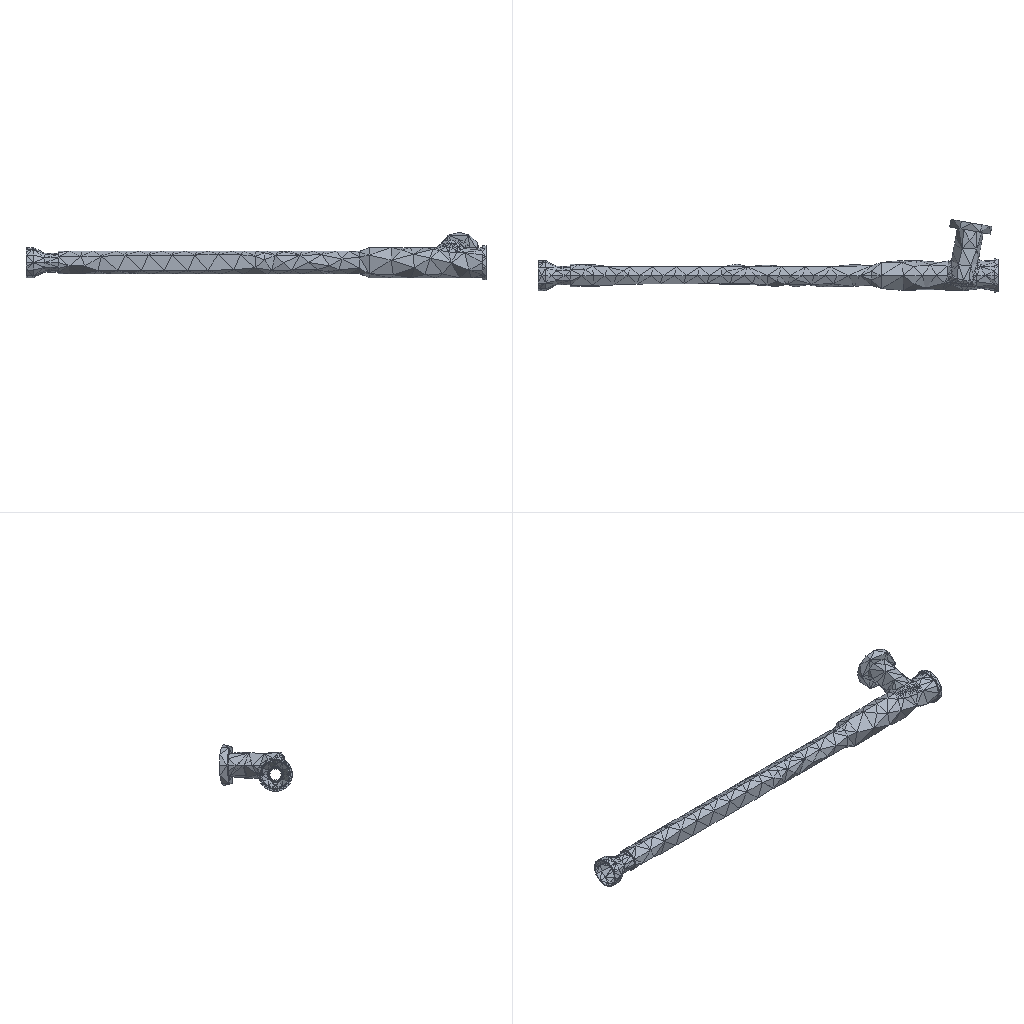Simulation study | ansys workbench
Ansys APDL input file, long lists of numbers shortened:
/batch
/config,noeldb,1     ! force off writing results to database
*get,_wallstrt,active,,time,wall
! ANSYS input file written by Workbench version 2022 R1
! File used for geometry attach: F:\ansys（分析文件汇总)\ansys转向器有限元分析\转向器\分析\齿轮轴.STEP
/title,wbnew--__ (C5)
! ****** Begin Custom Load Command Snippet ******
/COM, ACT Extensions:
/COM,     LSDYNA, 2021.1
/COM,
! ****** End   Custom Load Command Snippet ******
*DIM,_wb_ProjectScratch_dir,string,248
_wb_ProjectScratch_dir(1) = 'C:\Users\Administrator\AppData\Local\Temp\WB_Administrator_18756_2\_ProjectScratch\Scr9CF5\'
*DIM,_wb_SolverFiles_dir,string,248
_wb_SolverFiles_dir(1) = 'C:\Users\Administrator\AppData\Local\Temp\WB_Administrator_18756_2\wbnew_files\dp0\SYS-4\MECH\'
*DIM,_wb_userfiles_dir,string,248
_wb_userfiles_dir(1) = 'C:\Users\Administrator\AppData\Local\Temp\WB_Administrator_18756_2\wbnew_files\user_files\'
/com,--- Data in consistent NMM units. See Solving Units in the help system for more information.
/units,MPA
/nopr
/wb,file,start              !  signify a WB generated input file
/prep7
! Turn off shape checking because checks already performed inside WB mesher.
! See help system for more information.
SHPP,OFF,,NOWARN
/nolist
etcon,set             ! allow ANSYS to choose best KEYOP's for 180x elements, resets any applicable keyopt to MAPDL defaults
/com,*********** Nodes for the whole assembly ***********
nblock,3,,14898
(1i9,3e20.9e3)
        1     0.000000000E+00     1.290000000E+02    -2.000000000E+01
! (13543 more lines like these left out)
-1
/com,*********** Nodes for all Remote Points ***********
nblock,3
(1i9,3e20.9e3)
    13545    -4.024558464E-16     1.874095711E+02     4.440892099E-16
-1
/wb,elem,start            !  set before creation of elements
/com,*********** Elements for Body 1 "___-FreeParts|__-__1" ***********
et,1,187
eblock,19,solid,,7138
(19i9)
        1        1        1        1        0        0        0        0       10        0        1     1930     2216     2013     2164    12446    12852    12443    12445
! (14275 more lines like these left out)
-1
/wb,elem,end               !  done creating elements
/com,*********** Send User Defined Coordinate System(s) ***********
csys,0
toffst,273.15,  ! Temperature offset from absolute zero
/com,*********** Set Reference Temperature ***********
tref,22.
/wb,mat,start              !  starting to send materials
/com,*********** Send Materials ***********
Temperature = 'TEMP' ! Temperature
MP,DENS,1,7.85e-09,	! tonne mm^-3
MP,ALPX,1,1.2e-05,	! C^-1
MP,C,1,434000000,	! mm^2 s^-2 C^-1
MP,KXX,1,60.5,	! tonne mm s^-3 C^-1
MP,RSVX,1,0.00017,	! ohm mm
MP,EX,1,200000,	! tonne s^-2 mm^-1
MP,NUXY,1,0.3,
MP,MURX,1,10000,
/wb,mat,end                !  done sending materials
!************************* Model Summary ********************
!___-FreeParts|__-__1,	结构钢,	matid,	1
!************************* End Model Summary ********************
! get the diagonal of the bounding box. Needed later for other things
*get,_xmin,node,,mnloc,x
*get,_ymin,node,,mnloc,y
*get,_zmin,node,,mnloc,z
*get,_xmax,node,,mxloc,x
*get,_ymax,node,,mxloc,y
*get,_zmax,node,,mxloc,z
_ASMDIAG=(_xmax-_xmin)*(_xmax-_xmin)+(_ymax-_ymin)*(_ymax-_ymin)+(_zmax-_zmin)*(_zmax-_zmin)
_ASMDIAG=SQRT(_ASMDIAG)
/wb,contact,start          !  starting to send contact
/wb,contact,end            !  done creating contacts
/com,*********** Send Named Selection as Node Component ***********
CMBLOCK,______  ,NODE,     4510
(8i10)
        56        57        58        59        60        61        62        63
! (563 more lines like these left out)
/golist
/wb,load,start             !  starting to send loads
/gst,on,on
fini
*get,_numnode,node,0,count
*get,_numelem,elem,0,count
*get, _MAXELEMNUM, elem, 0, NUM, MAX
*get, _MAXNODENUM, node, 0, NUM, MAX
*get, _MAXELEMTYPE, etyp, 0, NUM, MAX
*get, _MAXREALCONST, real, 0, NUM, MAX
/go
/wb,load,end               !  done creating loads
/com,--- Number of total nodes = %_numnode%
/com,--- Number of contact elements = 0
/com,--- Number of spring elements = 0
/com,--- Number of bearing elements = 0
/com,--- Number of solid elements = 7138
/com,--- Number of condensed parts = 0
/com,--- Number of total elements = %_numelem%
*get,_wallbsol,active,,time,wall
/solu
antype,2                   ! modal analysis
_thickRatio=  1     ! Ratio of thick parts in the model
modopt,lanb,6
outres,erase
outres,all,none
outres,nsol,all
outres,etmp,all
mxpand                    ! default expand in case of complex solution
dmpopt,esav,no
dmpopt,emat,no
dmpopt,full,no
! *********** WB SOLVE COMMAND ***********
! check interactive state
*get,ANSINTER_,active,,int
*if,ANSINTER_,ne,0,then
/eof
*endif
solve
/com *************** Write FE CONNECTORS *********
CEWRITE,file,ce,,INTE
*get,_nmodalsolproc,active,0,numcpu
fini
/nopr
*get,_numnode,node,0,count
*get,_numelem,elem,0,count
*get, _MAXELEMNUM, elem, 0, NUM, MAX
*get, _MAXNODENUM, node, 0, NUM, MAX,,,INTERNAL
*get, _MAXELEMTYPE, etyp, 0, NUM, MAX
*get, _MAXREALCONST, real, 0, NUM, MAX
/gopr
*get,_wallasol,active,,time,wall
/post1
/nopr
*dim,_direction,CHAR,6,1
_direction(1) = 'X'
_direction(2) = 'Y'
_direction(3) = 'Z'
_direction(4) = 'ROTX'
_direction(5) = 'ROTY'
_direction(6) = 'ROTZ'
*get,_lastLS,active,0,set,LSTP
*get,_beginset,active,0,set,nset,first,_lastLS
*get,_endset,active,0,set,nset,last,_lastLS
_nummodes = 0
*if,_endset,gt,0,then
_nummodes = _endset - _beginset + 1
*endif
*do,i_mode,1,_nummodes
   *do,j_component,1,6
			*get,PFACT_%i_mode%_%j_component%,MODE,%i_mode%,PFACT,,DIREC,_direction(%j_component%)
   *enddo
*enddo
*dim,_tmdirection,CHAR,6,1
_tmdirection(1) = 'X'
_tmdirection(2) = 'Y'
_tmdirection(3) = 'Z'
_tmdirection(4) = 'X'
_tmdirection(5) = 'Y'
_tmdirection(6) = 'Z'
*do,j_component,1,6
    *if,j_component,gt,3,then
        *get,TOTALMASS_%j_component%,ELEM,0,IOR,_tmdirection(%j_component%)
    *else
        *get,TOTALMASS_%j_component%,ELEM,0,MTOT,_tmdirection(%j_component%)
    *endif
*enddo
/gopr
xmlo,ENCODING,ISO-8859-1
xmlo,parm
/xml,parm,xml
fini
/gopr
*get,_walldone,active,,time,wall
_preptime=(_wallbsol-_wallstrt)*3600
_solvtime=(_wallasol-_wallbsol)*3600
_posttime=(_walldone-_wallasol)*3600
_totaltim=(_walldone-_wallstrt)*3600
*get,_dlbratio,active,0,solu,dlbr
*get,_combtime,active,0,solu,comb
*get,_ssmode,active,0,solu,ssmm
*get,_ndofs,active,0,solu,ndof
/fclean				!clean distributed files
/com,--- Total number of nodes = %_numnode%
/com,--- Total number of elements = %_numelem%
/com,--- Element load balance ratio = %_dlbratio%
/com,--- Time to combine distributed files = %_combtime%
/com,--- Sparse memory mode = %_ssmode%
/com,--- Number of DOF = %_ndofs%
/wb,file,end               ! done with WB generated input